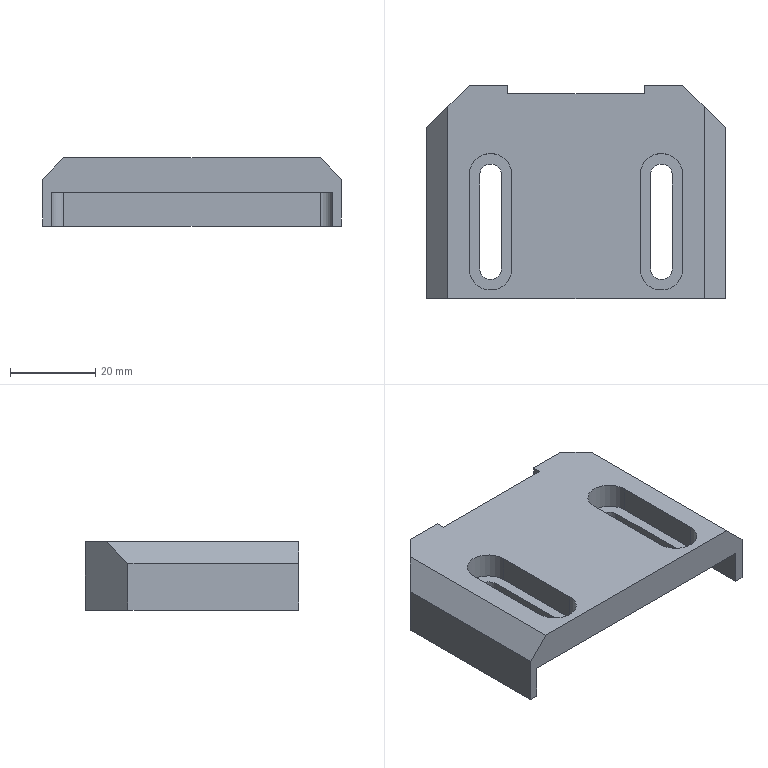Part | SolidWorks | features ICE 4, Chamfer 2, Extrusion 1, HoleWzd 1 | 1 solid | 46 faces | box 70 x 50 x 16 mm | volume 29528 mm3 | plane 28 | cylinder 14 | cone 4 | commonest cylinder face diameters 4.2 x4 5.1 x4 10 x4 6 x2
STEP:
#1=CARTESIAN_POINT('',(-10.,14.6,-2.1));
#2=VERTEX_POINT('',#1);
#3=CARTESIAN_POINT('',(-10.,14.6,2.1));
#4=VERTEX_POINT('',#3);
#5=CARTESIAN_POINT('',(-10.,14.6,0.));
#6=DIRECTION('',(0.,1.,0.));
#7=DIRECTION('',(0.,0.,1.));
#8=AXIS2_PLACEMENT_3D('',#5,#6,#7);
#9=CIRCLE('',#8,2.1);
#10=EDGE_CURVE('',#2,#4,#9,.T.);
#11=ORIENTED_EDGE('',*,*,#10,.F.);
#12=CARTESIAN_POINT('',(-10.,23.,-2.1));
#13=VERTEX_POINT('',#12);
#14=CARTESIAN_POINT('',(-10.,23.,-2.1));
#15=DIRECTION('',(0.,1.,0.));
#16=VECTOR('',#15,1000.);
#17=LINE('',#14,#16);
#18=EDGE_CURVE('',#2,#13,#17,.T.);
#19=ORIENTED_EDGE('',*,*,#18,.T.);
#20=CARTESIAN_POINT('',(-10.,23.,2.1));
#21=VERTEX_POINT('',#20);
#22=CARTESIAN_POINT('',(-10.,23.,0.));
#23=DIRECTION('',(0.,1.,0.));
#24=DIRECTION('',(0.,0.,1.));
#25=AXIS2_PLACEMENT_3D('',#22,#23,#24);
#26=CIRCLE('',#25,2.1);
#27=EDGE_CURVE('',#13,#21,#26,.T.);
#28=ORIENTED_EDGE('',*,*,#27,.T.);
#29=CARTESIAN_POINT('',(-10.,23.,2.1));
#30=DIRECTION('',(0.,1.,0.));
#31=VECTOR('',#30,1000.);
#32=LINE('',#29,#31);
#33=EDGE_CURVE('',#4,#21,#32,.T.);
#34=ORIENTED_EDGE('',*,*,#33,.F.);
#35=EDGE_LOOP('',(#11,#19,#28,#34));
#36=FACE_OUTER_BOUND('',#35,.T.);
#37=CARTESIAN_POINT('',(-10.,23.,0.));
#38=DIRECTION('',(0.,1.,0.));
#39=DIRECTION('',(0.,0.,1.));
#40=AXIS2_PLACEMENT_3D('',#37,#38,#39);
#41=CYLINDRICAL_SURFACE('',#40,2.1);
#42=ADVANCED_FACE('',(#36),#41,.F.);
#43=CARTESIAN_POINT('',(-10.,13.338,0.));
#44=VERTEX_POINT('',#43);
#45=CARTESIAN_POINT('',(-10.,14.6,2.1));
#46=DIRECTION('',(0.,0.515,0.8572));
#47=VECTOR('',#46,1000.);
#48=LINE('',#45,#47);
#49=EDGE_CURVE('',#44,#4,#48,.T.);
#50=ORIENTED_EDGE('',*,*,#49,.F.);
#51=CARTESIAN_POINT('',(-10.,14.6,-2.1));
#52=DIRECTION('',(0.,0.515,-0.8572));
#53=VECTOR('',#52,1000.);
#54=LINE('',#51,#53);
#55=EDGE_CURVE('',#44,#2,#54,.T.);
#56=ORIENTED_EDGE('',*,*,#55,.T.);
#57=ORIENTED_EDGE('',*,*,#10,.T.);
#58=EDGE_LOOP('',(#50,#56,#57));
#59=FACE_OUTER_BOUND('',#58,.T.);
#60=CARTESIAN_POINT('',(-10.,14.6,0.));
#61=DIRECTION('',(0.,1.,0.));
#62=DIRECTION('',(0.,0.,1.));
#63=AXIS2_PLACEMENT_3D('',#60,#61,#62);
#64=CONICAL_SURFACE('',#63,2.1,1.03);
#65=ADVANCED_FACE('',(#59),#64,.F.);
#66=CARTESIAN_POINT('',(10.,14.6,-2.1));
#67=VERTEX_POINT('',#66);
#68=CARTESIAN_POINT('',(10.,14.6,2.1));
#69=VERTEX_POINT('',#68);
#70=CARTESIAN_POINT('',(10.,14.6,0.));
#71=DIRECTION('',(0.,1.,0.));
#72=DIRECTION('',(0.,0.,1.));
#73=AXIS2_PLACEMENT_3D('',#70,#71,#72);
#74=CIRCLE('',#73,2.1);
#75=EDGE_CURVE('',#67,#69,#74,.T.);
#76=ORIENTED_EDGE('',*,*,#75,.F.);
#77=CARTESIAN_POINT('',(10.,23.,-2.1));
#78=VERTEX_POINT('',#77);
#79=CARTESIAN_POINT('',(10.,23.,-2.1));
#80=DIRECTION('',(0.,1.,0.));
#81=VECTOR('',#80,1000.);
#82=LINE('',#79,#81);
#83=EDGE_CURVE('',#67,#78,#82,.T.);
#84=ORIENTED_EDGE('',*,*,#83,.T.);
#85=CARTESIAN_POINT('',(10.,23.,2.1));
#86=VERTEX_POINT('',#85);
#87=CARTESIAN_POINT('',(10.,23.,0.));
#88=DIRECTION('',(0.,1.,0.));
#89=DIRECTION('',(0.,0.,1.));
#90=AXIS2_PLACEMENT_3D('',#87,#88,#89);
#91=CIRCLE('',#90,2.1);
#92=EDGE_CURVE('',#78,#86,#91,.T.);
#93=ORIENTED_EDGE('',*,*,#92,.T.);
#94=CARTESIAN_POINT('',(10.,23.,2.1));
#95=DIRECTION('',(0.,1.,0.));
#96=VECTOR('',#95,1000.);
#97=LINE('',#94,#96);
#98=EDGE_CURVE('',#69,#86,#97,.T.);
#99=ORIENTED_EDGE('',*,*,#98,.F.);
#100=EDGE_LOOP('',(#76,#84,#93,#99));
#101=FACE_OUTER_BOUND('',#100,.T.);
#102=CARTESIAN_POINT('',(10.,23.,0.));
#103=DIRECTION('',(0.,1.,0.));
#104=DIRECTION('',(0.,0.,1.));
#105=AXIS2_PLACEMENT_3D('',#102,#103,#104);
#106=CYLINDRICAL_SURFACE('',#105,2.1);
#107=ADVANCED_FACE('',(#101),#106,.F.);
#108=CARTESIAN_POINT('',(10.,13.338,0.));
#109=VERTEX_POINT('',#108);
#110=CARTESIAN_POINT('',(10.,14.6,2.1));
#111=DIRECTION('',(0.,0.515,0.8572));
#112=VECTOR('',#111,1000.);
#113=LINE('',#110,#112);
#114=EDGE_CURVE('',#109,#69,#113,.T.);
#115=ORIENTED_EDGE('',*,*,#114,.F.);
#116=CARTESIAN_POINT('',(10.,14.6,-2.1));
#117=DIRECTION('',(0.,0.515,-0.8572));
#118=VECTOR('',#117,1000.);
#119=LINE('',#116,#118);
#120=EDGE_CURVE('',#109,#67,#119,.T.);
#121=ORIENTED_EDGE('',*,*,#120,.T.);
#122=ORIENTED_EDGE('',*,*,#75,.T.);
#123=EDGE_LOOP('',(#115,#121,#122));
#124=FACE_OUTER_BOUND('',#123,.T.);
#125=CARTESIAN_POINT('',(10.,14.6,0.));
#126=DIRECTION('',(0.,1.,0.));
#127=DIRECTION('',(0.,0.,1.));
#128=AXIS2_PLACEMENT_3D('',#125,#126,#127);
#129=CONICAL_SURFACE('',#128,2.1,1.03);
#130=ADVANCED_FACE('',(#124),#129,.F.);
#131=CARTESIAN_POINT('',(-17.45,-18.,2.));
#132=VERTEX_POINT('',#131);
#133=CARTESIAN_POINT('',(-22.55,-18.,2.));
#134=VERTEX_POINT('',#133);
#135=CARTESIAN_POINT('',(-20.,-18.,2.));
#136=DIRECTION('',(0.,0.,-1.));
#137=DIRECTION('',(1.,0.,0.));
#138=AXIS2_PLACEMENT_3D('',#135,#136,#137);
#139=CIRCLE('',#138,2.55);
#140=EDGE_CURVE('',#132,#134,#139,.T.);
#141=ORIENTED_EDGE('',*,*,#140,.F.);
#142=CARTESIAN_POINT('',(-17.45,-18.,0.));
#143=VERTEX_POINT('',#142);
#144=CARTESIAN_POINT('',(-17.45,-18.,-8.));
#145=DIRECTION('',(0.,0.,1.));
#146=VECTOR('',#145,1000.);
#147=LINE('',#144,#146);
#148=EDGE_CURVE('',#143,#132,#147,.T.);
#149=ORIENTED_EDGE('',*,*,#148,.F.);
#150=CARTESIAN_POINT('',(-22.55,-18.,0.));
#151=VERTEX_POINT('',#150);
#152=CARTESIAN_POINT('',(-20.,-18.,0.));
#153=DIRECTION('',(0.,0.,-1.));
#154=DIRECTION('',(-1.,0.,0.));
#155=AXIS2_PLACEMENT_3D('',#152,#153,#154);
#156=CIRCLE('',#155,2.55);
#157=EDGE_CURVE('',#143,#151,#156,.T.);
#158=ORIENTED_EDGE('',*,*,#157,.T.);
#159=CARTESIAN_POINT('',(-22.55,-18.,-8.));
#160=DIRECTION('',(0.,0.,1.));
#161=VECTOR('',#160,1000.);
#162=LINE('',#159,#161);
#163=EDGE_CURVE('',#151,#134,#162,.T.);
#164=ORIENTED_EDGE('',*,*,#163,.T.);
#165=EDGE_LOOP('',(#141,#149,#158,#164));
#166=FACE_OUTER_BOUND('',#165,.T.);
#167=CARTESIAN_POINT('',(-20.,-18.,-8.));
#168=DIRECTION('',(0.,0.,1.));
#169=DIRECTION('',(1.,0.,0.));
#170=AXIS2_PLACEMENT_3D('',#167,#168,#169);
#171=CYLINDRICAL_SURFACE('',#170,2.55);
#172=ADVANCED_FACE('',(#166),#171,.F.);
#173=CARTESIAN_POINT('',(-22.55,4.,2.));
#174=VERTEX_POINT('',#173);
#175=CARTESIAN_POINT('',(-22.55,-18.,2.));
#176=DIRECTION('',(0.,1.,0.));
#177=VECTOR('',#176,1000.);
#178=LINE('',#175,#177);
#179=EDGE_CURVE('',#134,#174,#178,.T.);
#180=ORIENTED_EDGE('',*,*,#179,.F.);
#181=ORIENTED_EDGE('',*,*,#163,.F.);
#182=CARTESIAN_POINT('',(-22.55,4.,0.));
#183=VERTEX_POINT('',#182);
#184=CARTESIAN_POINT('',(-22.55,7.,0.));
#185=DIRECTION('',(0.,1.,0.));
#186=VECTOR('',#185,1000.);
#187=LINE('',#184,#186);
#188=EDGE_CURVE('',#151,#183,#187,.T.);
#189=ORIENTED_EDGE('',*,*,#188,.T.);
#190=CARTESIAN_POINT('',(-22.55,4.,-8.));
#191=DIRECTION('',(0.,0.,1.));
#192=VECTOR('',#191,1000.);
#193=LINE('',#190,#192);
#194=EDGE_CURVE('',#183,#174,#193,.T.);
#195=ORIENTED_EDGE('',*,*,#194,.T.);
#196=EDGE_LOOP('',(#180,#181,#189,#195));
#197=FACE_OUTER_BOUND('',#196,.T.);
#198=CARTESIAN_POINT('',(-22.55,-18.,-8.));
#199=DIRECTION('',(-1.,0.,0.));
#200=DIRECTION('',(0.,-1.,0.));
#201=AXIS2_PLACEMENT_3D('',#198,#199,#200);
#202=PLANE('',#201);
#203=ADVANCED_FACE('',(#197),#202,.F.);
#204=CARTESIAN_POINT('',(-17.45,4.,2.));
#205=VERTEX_POINT('',#204);
#206=CARTESIAN_POINT('',(-20.,4.,2.));
#207=DIRECTION('',(0.,0.,-1.));
#208=DIRECTION('',(1.,0.,0.));
#209=AXIS2_PLACEMENT_3D('',#206,#207,#208);
#210=CIRCLE('',#209,2.55);
#211=EDGE_CURVE('',#174,#205,#210,.T.);
#212=ORIENTED_EDGE('',*,*,#211,.F.);
#213=ORIENTED_EDGE('',*,*,#194,.F.);
#214=CARTESIAN_POINT('',(-17.45,4.,0.));
#215=VERTEX_POINT('',#214);
#216=CARTESIAN_POINT('',(-20.,4.,0.));
#217=DIRECTION('',(0.,0.,-1.));
#218=DIRECTION('',(-1.,0.,0.));
#219=AXIS2_PLACEMENT_3D('',#216,#217,#218);
#220=CIRCLE('',#219,2.55);
#221=EDGE_CURVE('',#183,#215,#220,.T.);
#222=ORIENTED_EDGE('',*,*,#221,.T.);
#223=CARTESIAN_POINT('',(-17.45,4.,-8.));
#224=DIRECTION('',(0.,0.,1.));
#225=VECTOR('',#224,1000.);
#226=LINE('',#223,#225);
#227=EDGE_CURVE('',#215,#205,#226,.T.);
#228=ORIENTED_EDGE('',*,*,#227,.T.);
#229=EDGE_LOOP('',(#212,#213,#222,#228));
#230=FACE_OUTER_BOUND('',#229,.T.);
#231=CARTESIAN_POINT('',(-20.,4.,-8.));
#232=DIRECTION('',(0.,0.,1.));
#233=DIRECTION('',(1.,0.,0.));
#234=AXIS2_PLACEMENT_3D('',#231,#232,#233);
#235=CYLINDRICAL_SURFACE('',#234,2.55);
#236=ADVANCED_FACE('',(#230),#235,.F.);
#237=CARTESIAN_POINT('',(-17.45,-18.,2.));
#238=DIRECTION('',(0.,-1.,0.));
#239=VECTOR('',#238,1000.);
#240=LINE('',#237,#239);
#241=EDGE_CURVE('',#205,#132,#240,.T.);
#242=ORIENTED_EDGE('',*,*,#241,.F.);
#243=ORIENTED_EDGE('',*,*,#227,.F.);
#244=CARTESIAN_POINT('',(-17.45,7.,0.));
#245=DIRECTION('',(0.,-1.,0.));
#246=VECTOR('',#245,1000.);
#247=LINE('',#244,#246);
#248=EDGE_CURVE('',#215,#143,#247,.T.);
#249=ORIENTED_EDGE('',*,*,#248,.T.);
#250=ORIENTED_EDGE('',*,*,#148,.T.);
#251=EDGE_LOOP('',(#242,#243,#249,#250));
#252=FACE_OUTER_BOUND('',#251,.T.);
#253=CARTESIAN_POINT('',(-17.45,-18.,-8.));
#254=DIRECTION('',(1.,0.,0.));
#255=DIRECTION('',(0.,1.,0.));
#256=AXIS2_PLACEMENT_3D('',#253,#254,#255);
#257=PLANE('',#256);
#258=ADVANCED_FACE('',(#252),#257,.F.);
#259=CARTESIAN_POINT('',(22.55,-18.,2.));
#260=VERTEX_POINT('',#259);
#261=CARTESIAN_POINT('',(17.45,-18.,2.));
#262=VERTEX_POINT('',#261);
#263=CARTESIAN_POINT('',(20.,-18.,2.));
#264=DIRECTION('',(0.,0.,-1.));
#265=DIRECTION('',(1.,0.,0.));
#266=AXIS2_PLACEMENT_3D('',#263,#264,#265);
#267=CIRCLE('',#266,2.55);
#268=EDGE_CURVE('',#260,#262,#267,.T.);
#269=ORIENTED_EDGE('',*,*,#268,.F.);
#270=CARTESIAN_POINT('',(22.55,-18.,0.));
#271=VERTEX_POINT('',#270);
#272=CARTESIAN_POINT('',(22.55,-18.,-8.));
#273=DIRECTION('',(0.,0.,1.));
#274=VECTOR('',#273,1000.);
#275=LINE('',#272,#274);
#276=EDGE_CURVE('',#271,#260,#275,.T.);
#277=ORIENTED_EDGE('',*,*,#276,.F.);
#278=CARTESIAN_POINT('',(17.45,-18.,0.));
#279=VERTEX_POINT('',#278);
#280=CARTESIAN_POINT('',(20.,-18.,0.));
#281=DIRECTION('',(0.,0.,-1.));
#282=DIRECTION('',(-1.,0.,0.));
#283=AXIS2_PLACEMENT_3D('',#280,#281,#282);
#284=CIRCLE('',#283,2.55);
#285=EDGE_CURVE('',#271,#279,#284,.T.);
#286=ORIENTED_EDGE('',*,*,#285,.T.);
#287=CARTESIAN_POINT('',(17.45,-18.,-8.));
#288=DIRECTION('',(0.,0.,1.));
#289=VECTOR('',#288,1000.);
#290=LINE('',#287,#289);
#291=EDGE_CURVE('',#279,#262,#290,.T.);
#292=ORIENTED_EDGE('',*,*,#291,.T.);
#293=EDGE_LOOP('',(#269,#277,#286,#292));
#294=FACE_OUTER_BOUND('',#293,.T.);
#295=CARTESIAN_POINT('',(20.,-18.,-8.));
#296=DIRECTION('',(0.,0.,1.));
#297=DIRECTION('',(1.,0.,0.));
#298=AXIS2_PLACEMENT_3D('',#295,#296,#297);
#299=CYLINDRICAL_SURFACE('',#298,2.55);
#300=ADVANCED_FACE('',(#294),#299,.F.);
#301=CARTESIAN_POINT('',(17.45,4.,2.));
#302=VERTEX_POINT('',#301);
#303=CARTESIAN_POINT('',(17.45,-18.,2.));
#304=DIRECTION('',(0.,1.,0.));
#305=VECTOR('',#304,1000.);
#306=LINE('',#303,#305);
#307=EDGE_CURVE('',#262,#302,#306,.T.);
#308=ORIENTED_EDGE('',*,*,#307,.F.);
#309=ORIENTED_EDGE('',*,*,#291,.F.);
#310=CARTESIAN_POINT('',(17.45,4.,0.));
#311=VERTEX_POINT('',#310);
#312=CARTESIAN_POINT('',(17.45,7.,0.));
#313=DIRECTION('',(0.,1.,0.));
#314=VECTOR('',#313,1000.);
#315=LINE('',#312,#314);
#316=EDGE_CURVE('',#279,#311,#315,.T.);
#317=ORIENTED_EDGE('',*,*,#316,.T.);
#318=CARTESIAN_POINT('',(17.45,4.,-8.));
#319=DIRECTION('',(0.,0.,1.));
#320=VECTOR('',#319,1000.);
#321=LINE('',#318,#320);
#322=EDGE_CURVE('',#311,#302,#321,.T.);
#323=ORIENTED_EDGE('',*,*,#322,.T.);
#324=EDGE_LOOP('',(#308,#309,#317,#323));
#325=FACE_OUTER_BOUND('',#324,.T.);
#326=CARTESIAN_POINT('',(17.45,-18.,-8.));
#327=DIRECTION('',(-1.,0.,0.));
#328=DIRECTION('',(0.,0.,1.));
#329=AXIS2_PLACEMENT_3D('',#326,#327,#328);
#330=PLANE('',#329);
#331=ADVANCED_FACE('',(#325),#330,.F.);
#332=CARTESIAN_POINT('',(22.55,4.,2.));
#333=VERTEX_POINT('',#332);
#334=CARTESIAN_POINT('',(20.,4.,2.));
#335=DIRECTION('',(0.,0.,-1.));
#336=DIRECTION('',(1.,0.,0.));
#337=AXIS2_PLACEMENT_3D('',#334,#335,#336);
#338=CIRCLE('',#337,2.55);
#339=EDGE_CURVE('',#302,#333,#338,.T.);
#340=ORIENTED_EDGE('',*,*,#339,.F.);
#341=ORIENTED_EDGE('',*,*,#322,.F.);
#342=CARTESIAN_POINT('',(22.55,4.,0.));
#343=VERTEX_POINT('',#342);
#344=CARTESIAN_POINT('',(20.,4.,0.));
#345=DIRECTION('',(0.,0.,-1.));
#346=DIRECTION('',(-1.,0.,0.));
#347=AXIS2_PLACEMENT_3D('',#344,#345,#346);
#348=CIRCLE('',#347,2.55);
#349=EDGE_CURVE('',#311,#343,#348,.T.);
#350=ORIENTED_EDGE('',*,*,#349,.T.);
#351=CARTESIAN_POINT('',(22.55,4.,-8.));
#352=DIRECTION('',(0.,0.,1.));
#353=VECTOR('',#352,1000.);
#354=LINE('',#351,#353);
#355=EDGE_CURVE('',#343,#333,#354,.T.);
#356=ORIENTED_EDGE('',*,*,#355,.T.);
#357=EDGE_LOOP('',(#340,#341,#350,#356));
#358=FACE_OUTER_BOUND('',#357,.T.);
#359=CARTESIAN_POINT('',(20.,4.,-8.));
#360=DIRECTION('',(0.,0.,1.));
#361=DIRECTION('',(1.,0.,0.));
#362=AXIS2_PLACEMENT_3D('',#359,#360,#361);
#363=CYLINDRICAL_SURFACE('',#362,2.55);
#364=ADVANCED_FACE('',(#358),#363,.F.);
#365=CARTESIAN_POINT('',(22.55,-18.,2.));
#366=DIRECTION('',(0.,-1.,0.));
#367=VECTOR('',#366,1000.);
#368=LINE('',#365,#367);
#369=EDGE_CURVE('',#333,#260,#368,.T.);
#370=ORIENTED_EDGE('',*,*,#369,.F.);
#371=ORIENTED_EDGE('',*,*,#355,.F.);
#372=CARTESIAN_POINT('',(22.55,7.,0.));
#373=DIRECTION('',(0.,-1.,0.));
#374=VECTOR('',#373,1000.);
#375=LINE('',#372,#374);
#376=EDGE_CURVE('',#343,#271,#375,.T.);
#377=ORIENTED_EDGE('',*,*,#376,.T.);
#378=ORIENTED_EDGE('',*,*,#276,.T.);
#379=EDGE_LOOP('',(#370,#371,#377,#378));
#380=FACE_OUTER_BOUND('',#379,.T.);
#381=CARTESIAN_POINT('',(22.55,-18.,-8.));
#382=DIRECTION('',(1.,0.,0.));
#383=DIRECTION('',(0.,0.,-1.));
#384=AXIS2_PLACEMENT_3D('',#381,#382,#383);
#385=PLANE('',#384);
#386=ADVANCED_FACE('',(#380),#385,.F.);
#387=CARTESIAN_POINT('',(-30.,-25.,8.));
#388=VERTEX_POINT('',#387);
#389=CARTESIAN_POINT('',(30.,-25.,8.));
#390=VERTEX_POINT('',#389);
#391=CARTESIAN_POINT('',(35.,-25.,8.));
#392=DIRECTION('',(1.,0.,0.));
#393=VECTOR('',#392,1000.);
#394=LINE('',#391,#393);
#395=EDGE_CURVE('',#388,#390,#394,.T.);
#396=ORIENTED_EDGE('',*,*,#395,.F.);
#397=CARTESIAN_POINT('',(-35.,-25.,3.));
#398=VERTEX_POINT('',#397);
#399=CARTESIAN_POINT('',(-30.,-25.,8.));
#400=DIRECTION('',(-0.7071,0.,-0.7071));
#401=VECTOR('',#400,1000.);
#402=LINE('',#399,#401);
#403=EDGE_CURVE('',#388,#398,#402,.T.);
#404=ORIENTED_EDGE('',*,*,#403,.T.);
#405=CARTESIAN_POINT('',(-35.,-25.,-8.));
#406=VERTEX_POINT('',#405);
#407=CARTESIAN_POINT('',(-35.,-25.,8.));
#408=DIRECTION('',(0.,0.,-1.));
#409=VECTOR('',#408,1000.);
#410=LINE('',#407,#409);
#411=EDGE_CURVE('',#398,#406,#410,.T.);
#412=ORIENTED_EDGE('',*,*,#411,.T.);
#413=CARTESIAN_POINT('',(-33.,-25.,-8.));
#414=VERTEX_POINT('',#413);
#415=CARTESIAN_POINT('',(35.,-25.,-8.));
#416=DIRECTION('',(1.,0.,0.));
#417=VECTOR('',#416,1000.);
#418=LINE('',#415,#417);
#419=EDGE_CURVE('',#406,#414,#418,.T.);
#420=ORIENTED_EDGE('',*,*,#419,.T.);
#421=CARTESIAN_POINT('',(-33.,-25.,0.));
#422=VERTEX_POINT('',#421);
#423=CARTESIAN_POINT('',(-33.,-25.,0.));
#424=DIRECTION('',(0.,0.,-1.));
#425=VECTOR('',#424,1000.);
#426=LINE('',#423,#425);
#427=EDGE_CURVE('',#422,#414,#426,.T.);
#428=ORIENTED_EDGE('',*,*,#427,.F.);
#429=CARTESIAN_POINT('',(33.,-25.,0.));
#430=VERTEX_POINT('',#429);
#431=CARTESIAN_POINT('',(-33.,-25.,0.));
#432=DIRECTION('',(1.,0.,0.));
#433=VECTOR('',#432,1000.);
#434=LINE('',#431,#433);
#435=EDGE_CURVE('',#422,#430,#434,.T.);
#436=ORIENTED_EDGE('',*,*,#435,.T.);
#437=CARTESIAN_POINT('',(33.,-25.,-8.));
#438=VERTEX_POINT('',#437);
#439=CARTESIAN_POINT('',(33.,-25.,0.));
#440=DIRECTION('',(0.,0.,-1.));
#441=VECTOR('',#440,1000.);
#442=LINE('',#439,#441);
#443=EDGE_CURVE('',#430,#438,#442,.T.);
#444=ORIENTED_EDGE('',*,*,#443,.T.);
#445=CARTESIAN_POINT('',(35.,-25.,-8.));
#446=VERTEX_POINT('',#445);
#447=CARTESIAN_POINT('',(35.,-25.,-8.));
#448=DIRECTION('',(1.,0.,0.));
#449=VECTOR('',#448,1000.);
#450=LINE('',#447,#449);
#451=EDGE_CURVE('',#438,#446,#450,.T.);
#452=ORIENTED_EDGE('',*,*,#451,.T.);
#453=CARTESIAN_POINT('',(35.,-25.,3.));
#454=VERTEX_POINT('',#453);
#455=CARTESIAN_POINT('',(35.,-25.,8.));
#456=DIRECTION('',(0.,0.,-1.));
#457=VECTOR('',#456,1000.);
#458=LINE('',#455,#457);
#459=EDGE_CURVE('',#454,#446,#458,.T.);
#460=ORIENTED_EDGE('',*,*,#459,.F.);
#461=CARTESIAN_POINT('',(30.,-25.,8.));
#462=DIRECTION('',(-0.7071,0.,0.7071));
#463=VECTOR('',#462,1000.);
#464=LINE('',#461,#463);
#465=EDGE_CURVE('',#454,#390,#464,.T.);
#466=ORIENTED_EDGE('',*,*,#465,.T.);
#467=EDGE_LOOP('',(#396,#404,#412,#420,#428,#436,#444,#452,#460,#466));
#468=FACE_OUTER_BOUND('',#467,.T.);
#469=CARTESIAN_POINT('',(35.,-25.,8.));
#470=DIRECTION('',(0.,1.,0.));
#471=DIRECTION('',(-1.,0.,0.));
#472=AXIS2_PLACEMENT_3D('',#469,#470,#471);
#473=PLANE('',#472);
#474=ADVANCED_FACE('',(#468),#473,.F.);
#475=CARTESIAN_POINT('',(-35.,15.,-8.));
#476=VERTEX_POINT('',#475);
#477=CARTESIAN_POINT('',(-35.,-25.,-8.));
#478=DIRECTION('',(0.,-1.,0.));
#479=VECTOR('',#478,1000.);
#480=LINE('',#477,#479);
#481=EDGE_CURVE('',#476,#406,#480,.T.);
#482=ORIENTED_EDGE('',*,*,#481,.F.);
#483=CARTESIAN_POINT('',(-25.,25.,-8.));
#484=VERTEX_POINT('',#483);
#485=CARTESIAN_POINT('',(-35.,15.,-8.));
#486=DIRECTION('',(0.7071,0.7071,0.));
#487=VECTOR('',#486,1000.);
#488=LINE('',#485,#487);
#489=EDGE_CURVE('',#476,#484,#488,.T.);
#490=ORIENTED_EDGE('',*,*,#489,.T.);
#491=CARTESIAN_POINT('',(-16.,25.,-8.));
#492=VERTEX_POINT('',#491);
#493=CARTESIAN_POINT('',(35.,25.,-8.));
#494=DIRECTION('',(-1.,0.,0.));
#495=VECTOR('',#494,1000.);
#496=LINE('',#493,#495);
#497=EDGE_CURVE('',#492,#484,#496,.T.);
#498=ORIENTED_EDGE('',*,*,#497,.F.);
#499=CARTESIAN_POINT('',(-16.,23.,-8.));
#500=VERTEX_POINT('',#499);
#501=CARTESIAN_POINT('',(-16.,23.,-8.));
#502=DIRECTION('',(0.,1.,0.));
#503=VECTOR('',#502,1000.);
#504=LINE('',#501,#503);
#505=EDGE_CURVE('',#500,#492,#504,.T.);
#506=ORIENTED_EDGE('',*,*,#505,.F.);
#507=CARTESIAN_POINT('',(16.,23.,-8.));
#508=VERTEX_POINT('',#507);
#509=CARTESIAN_POINT('',(16.,23.,-8.));
#510=DIRECTION('',(-1.,0.,0.));
#511=VECTOR('',#510,1000.);
#512=LINE('',#509,#511);
#513=EDGE_CURVE('',#508,#500,#512,.T.);
#514=ORIENTED_EDGE('',*,*,#513,.F.);
#515=CARTESIAN_POINT('',(16.,25.,-8.));
#516=VERTEX_POINT('',#515);
#517=CARTESIAN_POINT('',(16.,23.,-8.));
#518=DIRECTION('',(0.,1.,0.));
#519=VECTOR('',#518,1000.);
#520=LINE('',#517,#519);
#521=EDGE_CURVE('',#508,#516,#520,.T.);
#522=ORIENTED_EDGE('',*,*,#521,.T.);
#523=CARTESIAN_POINT('',(25.,25.,-8.));
#524=VERTEX_POINT('',#523);
#525=CARTESIAN_POINT('',(35.,25.,-8.));
#526=DIRECTION('',(-1.,0.,0.));
#527=VECTOR('',#526,1000.);
#528=LINE('',#525,#527);
#529=EDGE_CURVE('',#524,#516,#528,.T.);
#530=ORIENTED_EDGE('',*,*,#529,.F.);
#531=CARTESIAN_POINT('',(35.,15.,-8.));
#532=VERTEX_POINT('',#531);
#533=CARTESIAN_POINT('',(25.,25.,-8.));
#534=DIRECTION('',(0.7071,-0.7071,0.));
#535=VECTOR('',#534,1000.);
#536=LINE('',#533,#535);
#537=EDGE_CURVE('',#524,#532,#536,.T.);
#538=ORIENTED_EDGE('',*,*,#537,.T.);
#539=CARTESIAN_POINT('',(35.,-25.,-8.));
#540=DIRECTION('',(0.,1.,0.));
#541=VECTOR('',#540,1000.);
#542=LINE('',#539,#541);
#543=EDGE_CURVE('',#446,#532,#542,.T.);
#544=ORIENTED_EDGE('',*,*,#543,.F.);
#545=ORIENTED_EDGE('',*,*,#451,.F.);
#546=CARTESIAN_POINT('',(33.,7.,-8.));
#547=VERTEX_POINT('',#546);
#548=CARTESIAN_POINT('',(33.,-25.,-8.));
#549=DIRECTION('',(0.,1.,0.));
#550=VECTOR('',#549,1000.);
#551=LINE('',#548,#550);
#552=EDGE_CURVE('',#438,#547,#551,.T.);
#553=ORIENTED_EDGE('',*,*,#552,.T.);
#554=CARTESIAN_POINT('',(30.,10.,-8.));
#555=VERTEX_POINT('',#554);
#556=CARTESIAN_POINT('',(30.,7.,-8.));
#557=DIRECTION('',(0.,0.,1.));
#558=DIRECTION('',(-1.,0.,0.));
#559=AXIS2_PLACEMENT_3D('',#556,#557,#558);
#560=CIRCLE('',#559,3.);
#561=EDGE_CURVE('',#547,#555,#560,.T.);
#562=ORIENTED_EDGE('',*,*,#561,.T.);
#563=CARTESIAN_POINT('',(-30.,10.,-8.));
#564=VERTEX_POINT('',#563);
#565=CARTESIAN_POINT('',(-30.,10.,-8.));
#566=DIRECTION('',(-1.,0.,0.));
#567=VECTOR('',#566,1000.);
#568=LINE('',#565,#567);
#569=EDGE_CURVE('',#555,#564,#568,.T.);
#570=ORIENTED_EDGE('',*,*,#569,.T.);
#571=CARTESIAN_POINT('',(-33.,7.,-8.));
#572=VERTEX_POINT('',#571);
#573=CARTESIAN_POINT('',(-30.,7.,-8.));
#574=DIRECTION('',(0.,0.,1.));
#575=DIRECTION('',(-1.,0.,0.));
#576=AXIS2_PLACEMENT_3D('',#573,#574,#575);
#577=CIRCLE('',#576,3.);
#578=EDGE_CURVE('',#564,#572,#577,.T.);
#579=ORIENTED_EDGE('',*,*,#578,.T.);
#580=CARTESIAN_POINT('',(-33.,-25.,-8.));
#581=DIRECTION('',(0.,-1.,0.));
#582=VECTOR('',#581,1000.);
#583=LINE('',#580,#582);
#584=EDGE_CURVE('',#572,#414,#583,.T.);
#585=ORIENTED_EDGE('',*,*,#584,.T.);
#586=ORIENTED_EDGE('',*,*,#419,.F.);
#587=EDGE_LOOP('',(#482,#490,#498,#506,#514,#522,#530,#538,#544,#545,#553,#562,#570,#579,#585,#586));
#588=FACE_OUTER_BOUND('',#587,.T.);
#589=CARTESIAN_POINT('',(0.,0.,-8.));
#590=DIRECTION('',(0.,0.,1.));
#591=DIRECTION('',(1.,0.,0.));
#592=AXIS2_PLACEMENT_3D('',#589,#590,#591);
#593=PLANE('',#592);
#594=ADVANCED_FACE('',(#588),#593,.F.);
#595=ORIENTED_EDGE('',*,*,#497,.T.);
#596=CARTESIAN_POINT('',(-25.,25.,8.));
#597=VERTEX_POINT('',#596);
#598=CARTESIAN_POINT('',(-25.,25.,8.));
#599=DIRECTION('',(0.,0.,1.));
#600=VECTOR('',#599,1000.);
#601=LINE('',#598,#600);
#602=EDGE_CURVE('',#484,#597,#601,.T.);
#603=ORIENTED_EDGE('',*,*,#602,.T.);
#604=CARTESIAN_POINT('',(-16.,25.,8.));
#605=VERTEX_POINT('',#604);
#606=CARTESIAN_POINT('',(35.,25.,8.));
#607=DIRECTION('',(-1.,0.,0.));
#608=VECTOR('',#607,1000.);
#609=LINE('',#606,#608);
#610=EDGE_CURVE('',#605,#597,#609,.T.);
#611=ORIENTED_EDGE('',*,*,#610,.F.);
#612=CARTESIAN_POINT('',(-16.,25.,8.));
#613=DIRECTION('',(0.,0.,1.));
#614=VECTOR('',#613,1000.);
#615=LINE('',#612,#614);
#616=EDGE_CURVE('',#492,#605,#615,.T.);
#617=ORIENTED_EDGE('',*,*,#616,.F.);
#618=EDGE_LOOP('',(#595,#603,#611,#617));
#619=FACE_OUTER_BOUND('',#618,.T.);
#620=CARTESIAN_POINT('',(35.,25.,8.));
#621=DIRECTION('',(0.,-1.,0.));
#622=DIRECTION('',(1.,0.,0.));
#623=AXIS2_PLACEMENT_3D('',#620,#621,#622);
#624=PLANE('',#623);
#625=ADVANCED_FACE('',(#619),#624,.F.);
#626=ORIENTED_EDGE('',*,*,#411,.F.);
#627=CARTESIAN_POINT('',(-35.,15.,3.));
#628=VERTEX_POINT('',#627);
#629=CARTESIAN_POINT('',(-35.,15.,3.));
#630=DIRECTION('',(0.,1.,0.));
#631=VECTOR('',#630,1000.);
#632=LINE('',#629,#631);
#633=EDGE_CURVE('',#398,#628,#632,.T.);
#634=ORIENTED_EDGE('',*,*,#633,.T.);
#635=CARTESIAN_POINT('',(-35.,15.,8.));
#636=DIRECTION('',(0.,0.,-1.));
#637=VECTOR('',#636,1000.);
#638=LINE('',#635,#637);
#639=EDGE_CURVE('',#628,#476,#638,.T.);
#640=ORIENTED_EDGE('',*,*,#639,.T.);
#641=ORIENTED_EDGE('',*,*,#481,.T.);
#642=EDGE_LOOP('',(#626,#634,#640,#641));
#643=FACE_OUTER_BOUND('',#642,.T.);
#644=CARTESIAN_POINT('',(-35.,-25.,8.));
#645=DIRECTION('',(1.,0.,0.));
#646=DIRECTION('',(0.,0.,-1.));
#647=AXIS2_PLACEMENT_3D('',#644,#645,#646);
#648=PLANE('',#647);
#649=ADVANCED_FACE('',(#643),#648,.F.);
#650=CARTESIAN_POINT('',(35.,15.,3.));
#651=VERTEX_POINT('',#650);
#652=CARTESIAN_POINT('',(35.,15.,8.));
#653=DIRECTION('',(0.,0.,1.));
#654=VECTOR('',#653,1000.);
#655=LINE('',#652,#654);
#656=EDGE_CURVE('',#532,#651,#655,.T.);
#657=ORIENTED_EDGE('',*,*,#656,.T.);
#658=CARTESIAN_POINT('',(35.,-25.,3.));
#659=DIRECTION('',(0.,-1.,0.));
#660=VECTOR('',#659,1000.);
#661=LINE('',#658,#660);
#662=EDGE_CURVE('',#651,#454,#661,.T.);
#663=ORIENTED_EDGE('',*,*,#662,.T.);
#664=ORIENTED_EDGE('',*,*,#459,.T.);
#665=ORIENTED_EDGE('',*,*,#543,.T.);
#666=EDGE_LOOP('',(#657,#663,#664,#665));
#667=FACE_OUTER_BOUND('',#666,.T.);
#668=CARTESIAN_POINT('',(35.,-25.,8.));
#669=DIRECTION('',(-1.,0.,0.));
#670=DIRECTION('',(0.,0.,1.));
#671=AXIS2_PLACEMENT_3D('',#668,#669,#670);
#672=PLANE('',#671);
#673=ADVANCED_FACE('',(#667),#672,.F.);
#674=CARTESIAN_POINT('',(25.,25.,8.));
#675=VERTEX_POINT('',#674);
#676=CARTESIAN_POINT('',(16.,25.,8.));
#677=VERTEX_POINT('',#676);
#678=CARTESIAN_POINT('',(35.,25.,8.));
#679=DIRECTION('',(-1.,0.,0.));
#680=VECTOR('',#679,1000.);
#681=LINE('',#678,#680);
#682=EDGE_CURVE('',#675,#677,#681,.T.);
#683=ORIENTED_EDGE('',*,*,#682,.F.);
#684=CARTESIAN_POINT('',(25.,25.,8.));
#685=DIRECTION('',(0.,0.,-1.));
#686=VECTOR('',#685,1000.);
#687=LINE('',#684,#686);
#688=EDGE_CURVE('',#675,#524,#687,.T.);
#689=ORIENTED_EDGE('',*,*,#688,.T.);
#690=ORIENTED_EDGE('',*,*,#529,.T.);
#691=CARTESIAN_POINT('',(16.,25.,8.));
#692=DIRECTION('',(0.,0.,-1.));
#693=VECTOR('',#692,1000.);
#694=LINE('',#691,#693);
#695=EDGE_CURVE('',#677,#516,#694,.T.);
#696=ORIENTED_EDGE('',*,*,#695,.F.);
#697=EDGE_LOOP('',(#683,#689,#690,#696));
#698=FACE_OUTER_BOUND('',#697,.T.);
#699=CARTESIAN_POINT('',(35.,25.,8.));
#700=DIRECTION('',(0.,-1.,0.));
#701=DIRECTION('',(1.,0.,0.));
#702=AXIS2_PLACEMENT_3D('',#699,#700,#701);
#703=PLANE('',#702);
#704=ADVANCED_FACE('',(#698),#703,.F.);
#705=CARTESIAN_POINT('',(-15.,4.,8.));
#706=VERTEX_POINT('',#705);
#707=CARTESIAN_POINT('',(-25.,4.,8.));
#708=VERTEX_POINT('',#707);
#709=CARTESIAN_POINT('',(-20.,4.,8.));
#710=DIRECTION('',(0.,0.,1.));
#711=DIRECTION('',(1.,0.,0.));
#712=AXIS2_PLACEMENT_3D('',#709,#710,#711);
#713=CIRCLE('',#712,5.);
#714=EDGE_CURVE('',#706,#708,#713,.T.);
#715=ORIENTED_EDGE('',*,*,#714,.F.);
#716=CARTESIAN_POINT('',(-15.,-18.,8.));
#717=VERTEX_POINT('',#716);
#718=CARTESIAN_POINT('',(-15.,4.,8.));
#719=DIRECTION('',(0.,1.,0.));
#720=VECTOR('',#719,1000.);
#721=LINE('',#718,#720);
#722=EDGE_CURVE('',#717,#706,#721,.T.);
#723=ORIENTED_EDGE('',*,*,#722,.F.);
#724=CARTESIAN_POINT('',(-25.,-18.,8.));
#725=VERTEX_POINT('',#724);
#726=CARTESIAN_POINT('',(-20.,-18.,8.));
#727=DIRECTION('',(0.,0.,1.));
#728=DIRECTION('',(1.,0.,0.));
#729=AXIS2_PLACEMENT_3D('',#726,#727,#728);
#730=CIRCLE('',#729,5.);
#731=EDGE_CURVE('',#725,#717,#730,.T.);
#732=ORIENTED_EDGE('',*,*,#731,.F.);
#733=CARTESIAN_POINT('',(-25.,4.,8.));
#734=DIRECTION('',(0.,-1.,0.));
#735=VECTOR('',#734,1000.);
#736=LINE('',#733,#735);
#737=EDGE_CURVE('',#708,#725,#736,.T.);
#738=ORIENTED_EDGE('',*,*,#737,.F.);
#739=EDGE_LOOP('',(#715,#723,#732,#738));
#740=FACE_BOUND('',#739,.T.);
#741=CARTESIAN_POINT('',(15.,-18.,8.));
#742=VERTEX_POINT('',#741);
#743=CARTESIAN_POINT('',(25.,-18.,8.));
#744=VERTEX_POINT('',#743);
#745=CARTESIAN_POINT('',(20.,-18.,8.));
#746=DIRECTION('',(0.,0.,1.));
#747=DIRECTION('',(1.,0.,0.));
#748=AXIS2_PLACEMENT_3D('',#745,#746,#747);
#749=CIRCLE('',#748,5.);
#750=EDGE_CURVE('',#742,#744,#749,.T.);
#751=ORIENTED_EDGE('',*,*,#750,.F.);
#752=CARTESIAN_POINT('',(15.,4.,8.));
#753=VERTEX_POINT('',#752);
#754=CARTESIAN_POINT('',(15.,-18.,8.));
#755=DIRECTION('',(0.,-1.,0.));
#756=VECTOR('',#755,1000.);
#757=LINE('',#754,#756);
#758=EDGE_CURVE('',#753,#742,#757,.T.);
#759=ORIENTED_EDGE('',*,*,#758,.F.);
#760=CARTESIAN_POINT('',(25.,4.,8.));
#761=VERTEX_POINT('',#760);
#762=CARTESIAN_POINT('',(20.,4.,8.));
#763=DIRECTION('',(0.,0.,1.));
#764=DIRECTION('',(1.,0.,0.));
#765=AXIS2_PLACEMENT_3D('',#762,#763,#764);
#766=CIRCLE('',#765,5.);
#767=EDGE_CURVE('',#761,#753,#766,.T.);
#768=ORIENTED_EDGE('',*,*,#767,.F.);
#769=CARTESIAN_POINT('',(25.,-18.,8.));
#770=DIRECTION('',(0.,1.,0.));
#771=VECTOR('',#770,1000.);
#772=LINE('',#769,#771);
#773=EDGE_CURVE('',#744,#761,#772,.T.);
#774=ORIENTED_EDGE('',*,*,#773,.F.);
#775=EDGE_LOOP('',(#751,#759,#768,#774));
#776=FACE_BOUND('',#775,.T.);
#777=CARTESIAN_POINT('',(-30.,20.,8.));
#778=VERTEX_POINT('',#777);
#779=CARTESIAN_POINT('',(-25.,25.,8.));
#780=DIRECTION('',(-0.7071,-0.7071,0.));
#781=VECTOR('',#780,1000.);
#782=LINE('',#779,#781);
#783=EDGE_CURVE('',#597,#778,#782,.T.);
#784=ORIENTED_EDGE('',*,*,#783,.T.);
#785=CARTESIAN_POINT('',(-30.,-25.,8.));
#786=DIRECTION('',(0.,-1.,0.));
#787=VECTOR('',#786,1000.);
#788=LINE('',#785,#787);
#789=EDGE_CURVE('',#778,#388,#788,.T.);
#790=ORIENTED_EDGE('',*,*,#789,.T.);
#791=ORIENTED_EDGE('',*,*,#395,.T.);
#792=CARTESIAN_POINT('',(30.,20.,8.));
#793=VERTEX_POINT('',#792);
#794=CARTESIAN_POINT('',(30.,15.,8.));
#795=DIRECTION('',(0.,1.,0.));
#796=VECTOR('',#795,1000.);
#797=LINE('',#794,#796);
#798=EDGE_CURVE('',#390,#793,#797,.T.);
#799=ORIENTED_EDGE('',*,*,#798,.T.);
#800=CARTESIAN_POINT('',(25.,25.,8.));
#801=DIRECTION('',(-0.7071,0.7071,0.));
#802=VECTOR('',#801,1000.);
#803=LINE('',#800,#802);
#804=EDGE_CURVE('',#793,#675,#803,.T.);
#805=ORIENTED_EDGE('',*,*,#804,.T.);
#806=ORIENTED_EDGE('',*,*,#682,.T.);
#807=CARTESIAN_POINT('',(16.,23.,8.));
#808=VERTEX_POINT('',#807);
#809=CARTESIAN_POINT('',(16.,23.,8.));
#810=DIRECTION('',(0.,1.,0.));
#811=VECTOR('',#810,1000.);
#812=LINE('',#809,#811);
#813=EDGE_CURVE('',#808,#677,#812,.T.);
#814=ORIENTED_EDGE('',*,*,#813,.F.);
#815=CARTESIAN_POINT('',(-16.,23.,8.));
#816=VERTEX_POINT('',#815);
#817=CARTESIAN_POINT('',(16.,23.,8.));
#818=DIRECTION('',(1.,0.,0.));
#819=VECTOR('',#818,1000.);
#820=LINE('',#817,#819);
#821=EDGE_CURVE('',#816,#808,#820,.T.);
#822=ORIENTED_EDGE('',*,*,#821,.F.);
#823=CARTESIAN_POINT('',(-16.,23.,8.));
#824=DIRECTION('',(0.,1.,0.));
#825=VECTOR('',#824,1000.);
#826=LINE('',#823,#825);
#827=EDGE_CURVE('',#816,#605,#826,.T.);
#828=ORIENTED_EDGE('',*,*,#827,.T.);
#829=ORIENTED_EDGE('',*,*,#610,.T.);
#830=EDGE_LOOP('',(#784,#790,#791,#799,#805,#806,#814,#822,#828,#829));
#831=FACE_OUTER_BOUND('',#830,.T.);
#832=CARTESIAN_POINT('',(0.,0.,8.));
#833=DIRECTION('',(0.,0.,1.));
#834=DIRECTION('',(1.,0.,0.));
#835=AXIS2_PLACEMENT_3D('',#832,#833,#834);
#836=PLANE('',#835);
#837=ADVANCED_FACE('',(#740,#776,#831),#836,.T.);
#838=ORIENTED_EDGE('',*,*,#616,.T.);
#839=ORIENTED_EDGE('',*,*,#827,.F.);
#840=CARTESIAN_POINT('',(-16.,23.,8.));
#841=DIRECTION('',(0.,0.,1.));
#842=VECTOR('',#841,1000.);
#843=LINE('',#840,#842);
#844=EDGE_CURVE('',#500,#816,#843,.T.);
#845=ORIENTED_EDGE('',*,*,#844,.F.);
#846=ORIENTED_EDGE('',*,*,#505,.T.);
#847=EDGE_LOOP('',(#838,#839,#845,#846));
#848=FACE_OUTER_BOUND('',#847,.T.);
#849=CARTESIAN_POINT('',(-16.,23.,8.));
#850=DIRECTION('',(-1.,0.,0.));
#851=DIRECTION('',(0.,-1.,0.));
#852=AXIS2_PLACEMENT_3D('',#849,#850,#851);
#853=PLANE('',#852);
#854=ADVANCED_FACE('',(#848),#853,.F.);
#855=ORIENTED_EDGE('',*,*,#695,.T.);
#856=ORIENTED_EDGE('',*,*,#521,.F.);
#857=CARTESIAN_POINT('',(16.,23.,8.));
#858=DIRECTION('',(0.,0.,-1.));
#859=VECTOR('',#858,1000.);
#860=LINE('',#857,#859);
#861=EDGE_CURVE('',#808,#508,#860,.T.);
#862=ORIENTED_EDGE('',*,*,#861,.F.);
#863=ORIENTED_EDGE('',*,*,#813,.T.);
#864=EDGE_LOOP('',(#855,#856,#862,#863));
#865=FACE_OUTER_BOUND('',#864,.T.);
#866=CARTESIAN_POINT('',(16.,23.,8.));
#867=DIRECTION('',(1.,0.,0.));
#868=DIRECTION('',(0.,1.,0.));
#869=AXIS2_PLACEMENT_3D('',#866,#867,#868);
#870=PLANE('',#869);
#871=ADVANCED_FACE('',(#865),#870,.F.);
#872=CARTESIAN_POINT('',(-10.,23.,0.));
#873=DIRECTION('',(0.,1.,0.));
#874=DIRECTION('',(0.,0.,1.));
#875=AXIS2_PLACEMENT_3D('',#872,#873,#874);
#876=CIRCLE('',#875,2.1);
#877=EDGE_CURVE('',#21,#13,#876,.T.);
#878=ORIENTED_EDGE('',*,*,#877,.F.);
#879=ORIENTED_EDGE('',*,*,#27,.F.);
#880=EDGE_LOOP('',(#878,#879));
#881=FACE_BOUND('',#880,.T.);
#882=CARTESIAN_POINT('',(10.,23.,0.));
#883=DIRECTION('',(0.,1.,0.));
#884=DIRECTION('',(0.,0.,1.));
#885=AXIS2_PLACEMENT_3D('',#882,#883,#884);
#886=CIRCLE('',#885,2.1);
#887=EDGE_CURVE('',#86,#78,#886,.T.);
#888=ORIENTED_EDGE('',*,*,#887,.F.);
#889=ORIENTED_EDGE('',*,*,#92,.F.);
#890=EDGE_LOOP('',(#888,#889));
#891=FACE_BOUND('',#890,.T.);
#892=ORIENTED_EDGE('',*,*,#844,.T.);
#893=ORIENTED_EDGE('',*,*,#821,.T.);
#894=ORIENTED_EDGE('',*,*,#861,.T.);
#895=ORIENTED_EDGE('',*,*,#513,.T.);
#896=EDGE_LOOP('',(#892,#893,#894,#895));
#897=FACE_OUTER_BOUND('',#896,.T.);
#898=CARTESIAN_POINT('',(0.,23.,0.));
#899=DIRECTION('',(0.,1.,0.));
#900=DIRECTION('',(-1.,0.,0.));
#901=AXIS2_PLACEMENT_3D('',#898,#899,#900);
#902=PLANE('',#901);
#903=ADVANCED_FACE('',(#881,#891,#897),#902,.T.);
#904=ORIENTED_EDGE('',*,*,#120,.F.);
#905=ORIENTED_EDGE('',*,*,#114,.T.);
#906=CARTESIAN_POINT('',(10.,14.6,0.));
#907=DIRECTION('',(0.,1.,0.));
#908=DIRECTION('',(0.,0.,1.));
#909=AXIS2_PLACEMENT_3D('',#906,#907,#908);
#910=CIRCLE('',#909,2.1);
#911=EDGE_CURVE('',#69,#67,#910,.T.);
#912=ORIENTED_EDGE('',*,*,#911,.T.);
#913=EDGE_LOOP('',(#904,#905,#912));
#914=FACE_OUTER_BOUND('',#913,.T.);
#915=CARTESIAN_POINT('',(10.,14.6,0.));
#916=DIRECTION('',(0.,1.,0.));
#917=DIRECTION('',(0.,0.,1.));
#918=AXIS2_PLACEMENT_3D('',#915,#916,#917);
#919=CONICAL_SURFACE('',#918,2.1,1.03);
#920=ADVANCED_FACE('',(#914),#919,.F.);
#921=ORIENTED_EDGE('',*,*,#83,.F.);
#922=ORIENTED_EDGE('',*,*,#911,.F.);
#923=ORIENTED_EDGE('',*,*,#98,.T.);
#924=ORIENTED_EDGE('',*,*,#887,.T.);
#925=EDGE_LOOP('',(#921,#922,#923,#924));
#926=FACE_OUTER_BOUND('',#925,.T.);
#927=CARTESIAN_POINT('',(10.,23.,0.));
#928=DIRECTION('',(0.,1.,0.));
#929=DIRECTION('',(0.,0.,1.));
#930=AXIS2_PLACEMENT_3D('',#927,#928,#929);
#931=CYLINDRICAL_SURFACE('',#930,2.1);
#932=ADVANCED_FACE('',(#926),#931,.F.);
#933=ORIENTED_EDGE('',*,*,#55,.F.);
#934=ORIENTED_EDGE('',*,*,#49,.T.);
#935=CARTESIAN_POINT('',(-10.,14.6,0.));
#936=DIRECTION('',(0.,1.,0.));
#937=DIRECTION('',(0.,0.,1.));
#938=AXIS2_PLACEMENT_3D('',#935,#936,#937);
#939=CIRCLE('',#938,2.1);
#940=EDGE_CURVE('',#4,#2,#939,.T.);
#941=ORIENTED_EDGE('',*,*,#940,.T.);
#942=EDGE_LOOP('',(#933,#934,#941));
#943=FACE_OUTER_BOUND('',#942,.T.);
#944=CARTESIAN_POINT('',(-10.,14.6,0.));
#945=DIRECTION('',(0.,1.,0.));
#946=DIRECTION('',(0.,0.,1.));
#947=AXIS2_PLACEMENT_3D('',#944,#945,#946);
#948=CONICAL_SURFACE('',#947,2.1,1.03);
#949=ADVANCED_FACE('',(#943),#948,.F.);
#950=ORIENTED_EDGE('',*,*,#18,.F.);
#951=ORIENTED_EDGE('',*,*,#940,.F.);
#952=ORIENTED_EDGE('',*,*,#33,.T.);
#953=ORIENTED_EDGE('',*,*,#877,.T.);
#954=EDGE_LOOP('',(#950,#951,#952,#953));
#955=FACE_OUTER_BOUND('',#954,.T.);
#956=CARTESIAN_POINT('',(-10.,23.,0.));
#957=DIRECTION('',(0.,1.,0.));
#958=DIRECTION('',(0.,0.,1.));
#959=AXIS2_PLACEMENT_3D('',#956,#957,#958);
#960=CYLINDRICAL_SURFACE('',#959,2.1);
#961=ADVANCED_FACE('',(#955),#960,.F.);
#962=ORIENTED_EDGE('',*,*,#584,.F.);
#963=CARTESIAN_POINT('',(-33.,7.,0.));
#964=VERTEX_POINT('',#963);
#965=CARTESIAN_POINT('',(-33.,7.,0.));
#966=DIRECTION('',(0.,0.,-1.));
#967=VECTOR('',#966,1000.);
#968=LINE('',#965,#967);
#969=EDGE_CURVE('',#964,#572,#968,.T.);
#970=ORIENTED_EDGE('',*,*,#969,.F.);
#971=CARTESIAN_POINT('',(-33.,-25.,0.));
#972=DIRECTION('',(0.,-1.,0.));
#973=VECTOR('',#972,1000.);
#974=LINE('',#971,#973);
#975=EDGE_CURVE('',#964,#422,#974,.T.);
#976=ORIENTED_EDGE('',*,*,#975,.T.);
#977=ORIENTED_EDGE('',*,*,#427,.T.);
#978=EDGE_LOOP('',(#962,#970,#976,#977));
#979=FACE_OUTER_BOUND('',#978,.T.);
#980=CARTESIAN_POINT('',(-33.,-25.,0.));
#981=DIRECTION('',(1.,0.,0.));
#982=DIRECTION('',(0.,0.,-1.));
#983=AXIS2_PLACEMENT_3D('',#980,#981,#982);
#984=PLANE('',#983);
#985=ADVANCED_FACE('',(#979),#984,.T.);
#986=ORIENTED_EDGE('',*,*,#552,.F.);
#987=ORIENTED_EDGE('',*,*,#443,.F.);
#988=CARTESIAN_POINT('',(33.,7.,0.));
#989=VERTEX_POINT('',#988);
#990=CARTESIAN_POINT('',(33.,-25.,0.));
#991=DIRECTION('',(0.,1.,0.));
#992=VECTOR('',#991,1000.);
#993=LINE('',#990,#992);
#994=EDGE_CURVE('',#430,#989,#993,.T.);
#995=ORIENTED_EDGE('',*,*,#994,.T.);
#996=CARTESIAN_POINT('',(33.,7.,0.));
#997=DIRECTION('',(0.,0.,-1.));
#998=VECTOR('',#997,1000.);
#999=LINE('',#996,#998);
#1000=EDGE_CURVE('',#989,#547,#999,.T.);
#1001=ORIENTED_EDGE('',*,*,#1000,.T.);
#1002=EDGE_LOOP('',(#986,#987,#995,#1001));
#1003=FACE_OUTER_BOUND('',#1002,.T.);
#1004=CARTESIAN_POINT('',(33.,-25.,0.));
#1005=DIRECTION('',(-1.,0.,0.));
#1006=DIRECTION('',(0.,0.,1.));
#1007=AXIS2_PLACEMENT_3D('',#1004,#1005,#1006);
#1008=PLANE('',#1007);
#1009=ADVANCED_FACE('',(#1003),#1008,.T.);
#1010=ORIENTED_EDGE('',*,*,#561,.F.);
#1011=ORIENTED_EDGE('',*,*,#1000,.F.);
#1012=CARTESIAN_POINT('',(30.,10.,0.));
#1013=VERTEX_POINT('',#1012);
#1014=CARTESIAN_POINT('',(30.,7.,0.));
#1015=DIRECTION('',(0.,0.,1.));
#1016=DIRECTION('',(-1.,0.,0.));
#1017=AXIS2_PLACEMENT_3D('',#1014,#1015,#1016);
#1018=CIRCLE('',#1017,3.);
#1019=EDGE_CURVE('',#989,#1013,#1018,.T.);
#1020=ORIENTED_EDGE('',*,*,#1019,.T.);
#1021=CARTESIAN_POINT('',(30.,10.,0.));
#1022=DIRECTION('',(0.,0.,-1.));
#1023=VECTOR('',#1022,1000.);
#1024=LINE('',#1021,#1023);
#1025=EDGE_CURVE('',#1013,#555,#1024,.T.);
#1026=ORIENTED_EDGE('',*,*,#1025,.T.);
#1027=EDGE_LOOP('',(#1010,#1011,#1020,#1026));
#1028=FACE_OUTER_BOUND('',#1027,.T.);
#1029=CARTESIAN_POINT('',(30.,7.,0.));
#1030=DIRECTION('',(0.,0.,-1.));
#1031=DIRECTION('',(-1.,0.,0.));
#1032=AXIS2_PLACEMENT_3D('',#1029,#1030,#1031);
#1033=CYLINDRICAL_SURFACE('',#1032,3.);
#1034=ADVANCED_FACE('',(#1028),#1033,.F.);
#1035=ORIENTED_EDGE('',*,*,#569,.F.);
#1036=ORIENTED_EDGE('',*,*,#1025,.F.);
#1037=CARTESIAN_POINT('',(-30.,10.,0.));
#1038=VERTEX_POINT('',#1037);
#1039=CARTESIAN_POINT('',(-30.,10.,0.));
#1040=DIRECTION('',(-1.,0.,0.));
#1041=VECTOR('',#1040,1000.);
#1042=LINE('',#1039,#1041);
#1043=EDGE_CURVE('',#1013,#1038,#1042,.T.);
#1044=ORIENTED_EDGE('',*,*,#1043,.T.);
#1045=CARTESIAN_POINT('',(-30.,10.,0.));
#1046=DIRECTION('',(0.,0.,-1.));
#1047=VECTOR('',#1046,1000.);
#1048=LINE('',#1045,#1047);
#1049=EDGE_CURVE('',#1038,#564,#1048,.T.);
#1050=ORIENTED_EDGE('',*,*,#1049,.T.);
#1051=EDGE_LOOP('',(#1035,#1036,#1044,#1050));
#1052=FACE_OUTER_BOUND('',#1051,.T.);
#1053=CARTESIAN_POINT('',(-30.,10.,0.));
#1054=DIRECTION('',(0.,-1.,0.));
#1055=DIRECTION('',(0.,0.,-1.));
#1056=AXIS2_PLACEMENT_3D('',#1053,#1054,#1055);
#1057=PLANE('',#1056);
#1058=ADVANCED_FACE('',(#1052),#1057,.T.);
#1059=ORIENTED_EDGE('',*,*,#578,.F.);
#1060=ORIENTED_EDGE('',*,*,#1049,.F.);
#1061=CARTESIAN_POINT('',(-30.,7.,0.));
#1062=DIRECTION('',(0.,0.,1.));
#1063=DIRECTION('',(-1.,0.,0.));
#1064=AXIS2_PLACEMENT_3D('',#1061,#1062,#1063);
#1065=CIRCLE('',#1064,3.);
#1066=EDGE_CURVE('',#1038,#964,#1065,.T.);
#1067=ORIENTED_EDGE('',*,*,#1066,.T.);
#1068=ORIENTED_EDGE('',*,*,#969,.T.);
#1069=EDGE_LOOP('',(#1059,#1060,#1067,#1068));
#1070=FACE_OUTER_BOUND('',#1069,.T.);
#1071=CARTESIAN_POINT('',(-30.,7.,0.));
#1072=DIRECTION('',(0.,0.,-1.));
#1073=DIRECTION('',(-1.,0.,0.));
#1074=AXIS2_PLACEMENT_3D('',#1071,#1072,#1073);
#1075=CYLINDRICAL_SURFACE('',#1074,3.);
#1076=ADVANCED_FACE('',(#1070),#1075,.F.);
#1077=ORIENTED_EDGE('',*,*,#285,.F.);
#1078=ORIENTED_EDGE('',*,*,#376,.F.);
#1079=ORIENTED_EDGE('',*,*,#349,.F.);
#1080=ORIENTED_EDGE('',*,*,#316,.F.);
#1081=EDGE_LOOP('',(#1077,#1078,#1079,#1080));
#1082=FACE_BOUND('',#1081,.T.);
#1083=ORIENTED_EDGE('',*,*,#157,.F.);
#1084=ORIENTED_EDGE('',*,*,#248,.F.);
#1085=ORIENTED_EDGE('',*,*,#221,.F.);
#1086=ORIENTED_EDGE('',*,*,#188,.F.);
#1087=EDGE_LOOP('',(#1083,#1084,#1085,#1086));
#1088=FACE_BOUND('',#1087,.T.);
#1089=ORIENTED_EDGE('',*,*,#975,.F.);
#1090=ORIENTED_EDGE('',*,*,#1066,.F.);
#1091=ORIENTED_EDGE('',*,*,#1043,.F.);
#1092=ORIENTED_EDGE('',*,*,#1019,.F.);
#1093=ORIENTED_EDGE('',*,*,#994,.F.);
#1094=ORIENTED_EDGE('',*,*,#435,.F.);
#1095=EDGE_LOOP('',(#1089,#1090,#1091,#1092,#1093,#1094));
#1096=FACE_OUTER_BOUND('',#1095,.T.);
#1097=CARTESIAN_POINT('',(-30.,7.,0.));
#1098=DIRECTION('',(0.,0.,-1.));
#1099=DIRECTION('',(-1.,0.,0.));
#1100=AXIS2_PLACEMENT_3D('',#1097,#1098,#1099);
#1101=PLANE('',#1100);
#1102=ADVANCED_FACE('',(#1082,#1088,#1096),#1101,.T.);
#1103=CARTESIAN_POINT('',(15.,-18.,2.));
#1104=VERTEX_POINT('',#1103);
#1105=CARTESIAN_POINT('',(25.,-18.,2.));
#1106=VERTEX_POINT('',#1105);
#1107=CARTESIAN_POINT('',(20.,-18.,2.));
#1108=DIRECTION('',(0.,0.,1.));
#1109=DIRECTION('',(1.,0.,0.));
#1110=AXIS2_PLACEMENT_3D('',#1107,#1108,#1109);
#1111=CIRCLE('',#1110,5.);
#1112=EDGE_CURVE('',#1104,#1106,#1111,.T.);
#1113=ORIENTED_EDGE('',*,*,#1112,.T.);
#1114=CARTESIAN_POINT('',(25.,4.,2.));
#1115=VERTEX_POINT('',#1114);
#1116=CARTESIAN_POINT('',(25.,-18.,2.));
#1117=DIRECTION('',(0.,1.,0.));
#1118=VECTOR('',#1117,1000.);
#1119=LINE('',#1116,#1118);
#1120=EDGE_CURVE('',#1106,#1115,#1119,.T.);
#1121=ORIENTED_EDGE('',*,*,#1120,.T.);
#1122=CARTESIAN_POINT('',(15.,4.,2.));
#1123=VERTEX_POINT('',#1122);
#1124=CARTESIAN_POINT('',(20.,4.,2.));
#1125=DIRECTION('',(0.,0.,1.));
#1126=DIRECTION('',(1.,0.,0.));
#1127=AXIS2_PLACEMENT_3D('',#1124,#1125,#1126);
#1128=CIRCLE('',#1127,5.);
#1129=EDGE_CURVE('',#1115,#1123,#1128,.T.);
#1130=ORIENTED_EDGE('',*,*,#1129,.T.);
#1131=CARTESIAN_POINT('',(15.,-18.,2.));
#1132=DIRECTION('',(0.,-1.,0.));
#1133=VECTOR('',#1132,1000.);
#1134=LINE('',#1131,#1133);
#1135=EDGE_CURVE('',#1123,#1104,#1134,.T.);
#1136=ORIENTED_EDGE('',*,*,#1135,.T.);
#1137=EDGE_LOOP('',(#1113,#1121,#1130,#1136));
#1138=FACE_OUTER_BOUND('',#1137,.T.);
#1139=ORIENTED_EDGE('',*,*,#268,.T.);
#1140=ORIENTED_EDGE('',*,*,#307,.T.);
#1141=ORIENTED_EDGE('',*,*,#339,.T.);
#1142=ORIENTED_EDGE('',*,*,#369,.T.);
#1143=EDGE_LOOP('',(#1139,#1140,#1141,#1142));
#1144=FACE_BOUND('',#1143,.T.);
#1145=CARTESIAN_POINT('',(20.,-18.,2.));
#1146=DIRECTION('',(0.,0.,1.));
#1147=DIRECTION('',(1.,0.,0.));
#1148=AXIS2_PLACEMENT_3D('',#1145,#1146,#1147);
#1149=PLANE('',#1148);
#1150=ADVANCED_FACE('',(#1138,#1144),#1149,.T.);
#1151=ORIENTED_EDGE('',*,*,#750,.T.);
#1152=CARTESIAN_POINT('',(25.,-18.,2.));
#1153=DIRECTION('',(0.,0.,1.));
#1154=VECTOR('',#1153,1000.);
#1155=LINE('',#1152,#1154);
#1156=EDGE_CURVE('',#1106,#744,#1155,.T.);
#1157=ORIENTED_EDGE('',*,*,#1156,.F.);
#1158=ORIENTED_EDGE('',*,*,#1112,.F.);
#1159=CARTESIAN_POINT('',(15.,-18.,2.));
#1160=DIRECTION('',(0.,0.,1.));
#1161=VECTOR('',#1160,1000.);
#1162=LINE('',#1159,#1161);
#1163=EDGE_CURVE('',#1104,#742,#1162,.T.);
#1164=ORIENTED_EDGE('',*,*,#1163,.T.);
#1165=EDGE_LOOP('',(#1151,#1157,#1158,#1164));
#1166=FACE_OUTER_BOUND('',#1165,.T.);
#1167=CARTESIAN_POINT('',(20.,-18.,2.));
#1168=DIRECTION('',(0.,0.,1.));
#1169=DIRECTION('',(1.,0.,0.));
#1170=AXIS2_PLACEMENT_3D('',#1167,#1168,#1169);
#1171=CYLINDRICAL_SURFACE('',#1170,5.);
#1172=ADVANCED_FACE('',(#1166),#1171,.F.);
#1173=ORIENTED_EDGE('',*,*,#758,.T.);
#1174=ORIENTED_EDGE('',*,*,#1163,.F.);
#1175=ORIENTED_EDGE('',*,*,#1135,.F.);
#1176=CARTESIAN_POINT('',(15.,4.,2.));
#1177=DIRECTION('',(0.,0.,1.));
#1178=VECTOR('',#1177,1000.);
#1179=LINE('',#1176,#1178);
#1180=EDGE_CURVE('',#1123,#753,#1179,.T.);
#1181=ORIENTED_EDGE('',*,*,#1180,.T.);
#1182=EDGE_LOOP('',(#1173,#1174,#1175,#1181));
#1183=FACE_OUTER_BOUND('',#1182,.T.);
#1184=CARTESIAN_POINT('',(15.,-18.,2.));
#1185=DIRECTION('',(-1.,0.,0.));
#1186=DIRECTION('',(0.,0.,1.));
#1187=AXIS2_PLACEMENT_3D('',#1184,#1185,#1186);
#1188=PLANE('',#1187);
#1189=ADVANCED_FACE('',(#1183),#1188,.F.);
#1190=ORIENTED_EDGE('',*,*,#767,.T.);
#1191=ORIENTED_EDGE('',*,*,#1180,.F.);
#1192=ORIENTED_EDGE('',*,*,#1129,.F.);
#1193=CARTESIAN_POINT('',(25.,4.,2.));
#1194=DIRECTION('',(0.,0.,1.));
#1195=VECTOR('',#1194,1000.);
#1196=LINE('',#1193,#1195);
#1197=EDGE_CURVE('',#1115,#761,#1196,.T.);
#1198=ORIENTED_EDGE('',*,*,#1197,.T.);
#1199=EDGE_LOOP('',(#1190,#1191,#1192,#1198));
#1200=FACE_OUTER_BOUND('',#1199,.T.);
#1201=CARTESIAN_POINT('',(20.,4.,2.));
#1202=DIRECTION('',(0.,0.,1.));
#1203=DIRECTION('',(1.,0.,0.));
#1204=AXIS2_PLACEMENT_3D('',#1201,#1202,#1203);
#1205=CYLINDRICAL_SURFACE('',#1204,5.);
#1206=ADVANCED_FACE('',(#1200),#1205,.F.);
#1207=ORIENTED_EDGE('',*,*,#773,.T.);
#1208=ORIENTED_EDGE('',*,*,#1197,.F.);
#1209=ORIENTED_EDGE('',*,*,#1120,.F.);
#1210=ORIENTED_EDGE('',*,*,#1156,.T.);
#1211=EDGE_LOOP('',(#1207,#1208,#1209,#1210));
#1212=FACE_OUTER_BOUND('',#1211,.T.);
#1213=CARTESIAN_POINT('',(25.,-18.,2.));
#1214=DIRECTION('',(1.,0.,0.));
#1215=DIRECTION('',(0.,0.,-1.));
#1216=AXIS2_PLACEMENT_3D('',#1213,#1214,#1215);
#1217=PLANE('',#1216);
#1218=ADVANCED_FACE('',(#1212),#1217,.F.);
#1219=CARTESIAN_POINT('',(-15.,4.,2.));
#1220=VERTEX_POINT('',#1219);
#1221=CARTESIAN_POINT('',(-25.,4.,2.));
#1222=VERTEX_POINT('',#1221);
#1223=CARTESIAN_POINT('',(-20.,4.,2.));
#1224=DIRECTION('',(0.,0.,1.));
#1225=DIRECTION('',(1.,0.,0.));
#1226=AXIS2_PLACEMENT_3D('',#1223,#1224,#1225);
#1227=CIRCLE('',#1226,5.);
#1228=EDGE_CURVE('',#1220,#1222,#1227,.T.);
#1229=ORIENTED_EDGE('',*,*,#1228,.T.);
#1230=CARTESIAN_POINT('',(-25.,-18.,2.));
#1231=VERTEX_POINT('',#1230);
#1232=CARTESIAN_POINT('',(-25.,4.,2.));
#1233=DIRECTION('',(0.,-1.,0.));
#1234=VECTOR('',#1233,1000.);
#1235=LINE('',#1232,#1234);
#1236=EDGE_CURVE('',#1222,#1231,#1235,.T.);
#1237=ORIENTED_EDGE('',*,*,#1236,.T.);
#1238=CARTESIAN_POINT('',(-15.,-18.,2.));
#1239=VERTEX_POINT('',#1238);
#1240=CARTESIAN_POINT('',(-20.,-18.,2.));
#1241=DIRECTION('',(0.,0.,1.));
#1242=DIRECTION('',(1.,0.,0.));
#1243=AXIS2_PLACEMENT_3D('',#1240,#1241,#1242);
#1244=CIRCLE('',#1243,5.);
#1245=EDGE_CURVE('',#1231,#1239,#1244,.T.);
#1246=ORIENTED_EDGE('',*,*,#1245,.T.);
#1247=CARTESIAN_POINT('',(-15.,4.,2.));
#1248=DIRECTION('',(0.,1.,0.));
#1249=VECTOR('',#1248,1000.);
#1250=LINE('',#1247,#1249);
#1251=EDGE_CURVE('',#1239,#1220,#1250,.T.);
#1252=ORIENTED_EDGE('',*,*,#1251,.T.);
#1253=EDGE_LOOP('',(#1229,#1237,#1246,#1252));
#1254=FACE_OUTER_BOUND('',#1253,.T.);
#1255=ORIENTED_EDGE('',*,*,#140,.T.);
#1256=ORIENTED_EDGE('',*,*,#179,.T.);
#1257=ORIENTED_EDGE('',*,*,#211,.T.);
#1258=ORIENTED_EDGE('',*,*,#241,.T.);
#1259=EDGE_LOOP('',(#1255,#1256,#1257,#1258));
#1260=FACE_BOUND('',#1259,.T.);
#1261=CARTESIAN_POINT('',(-20.,4.,2.));
#1262=DIRECTION('',(0.,0.,1.));
#1263=DIRECTION('',(1.,0.,0.));
#1264=AXIS2_PLACEMENT_3D('',#1261,#1262,#1263);
#1265=PLANE('',#1264);
#1266=ADVANCED_FACE('',(#1254,#1260),#1265,.T.);
#1267=ORIENTED_EDGE('',*,*,#714,.T.);
#1268=CARTESIAN_POINT('',(-25.,4.,2.));
#1269=DIRECTION('',(0.,0.,1.));
#1270=VECTOR('',#1269,1000.);
#1271=LINE('',#1268,#1270);
#1272=EDGE_CURVE('',#1222,#708,#1271,.T.);
#1273=ORIENTED_EDGE('',*,*,#1272,.F.);
#1274=ORIENTED_EDGE('',*,*,#1228,.F.);
#1275=CARTESIAN_POINT('',(-15.,4.,2.));
#1276=DIRECTION('',(0.,0.,1.));
#1277=VECTOR('',#1276,1000.);
#1278=LINE('',#1275,#1277);
#1279=EDGE_CURVE('',#1220,#706,#1278,.T.);
#1280=ORIENTED_EDGE('',*,*,#1279,.T.);
#1281=EDGE_LOOP('',(#1267,#1273,#1274,#1280));
#1282=FACE_OUTER_BOUND('',#1281,.T.);
#1283=CARTESIAN_POINT('',(-20.,4.,2.));
#1284=DIRECTION('',(0.,0.,1.));
#1285=DIRECTION('',(1.,0.,0.));
#1286=AXIS2_PLACEMENT_3D('',#1283,#1284,#1285);
#1287=CYLINDRICAL_SURFACE('',#1286,5.);
#1288=ADVANCED_FACE('',(#1282),#1287,.F.);
#1289=ORIENTED_EDGE('',*,*,#722,.T.);
#1290=ORIENTED_EDGE('',*,*,#1279,.F.);
#1291=ORIENTED_EDGE('',*,*,#1251,.F.);
#1292=CARTESIAN_POINT('',(-15.,-18.,2.));
#1293=DIRECTION('',(0.,0.,1.));
#1294=VECTOR('',#1293,1000.);
#1295=LINE('',#1292,#1294);
#1296=EDGE_CURVE('',#1239,#717,#1295,.T.);
#1297=ORIENTED_EDGE('',*,*,#1296,.T.);
#1298=EDGE_LOOP('',(#1289,#1290,#1291,#1297));
#1299=FACE_OUTER_BOUND('',#1298,.T.);
#1300=CARTESIAN_POINT('',(-15.,4.,2.));
#1301=DIRECTION('',(1.,0.,0.));
#1302=DIRECTION('',(0.,0.,-1.));
#1303=AXIS2_PLACEMENT_3D('',#1300,#1301,#1302);
#1304=PLANE('',#1303);
#1305=ADVANCED_FACE('',(#1299),#1304,.F.);
#1306=ORIENTED_EDGE('',*,*,#731,.T.);
#1307=ORIENTED_EDGE('',*,*,#1296,.F.);
#1308=ORIENTED_EDGE('',*,*,#1245,.F.);
#1309=CARTESIAN_POINT('',(-25.,-18.,2.));
#1310=DIRECTION('',(0.,0.,1.));
#1311=VECTOR('',#1310,1000.);
#1312=LINE('',#1309,#1311);
#1313=EDGE_CURVE('',#1231,#725,#1312,.T.);
#1314=ORIENTED_EDGE('',*,*,#1313,.T.);
#1315=EDGE_LOOP('',(#1306,#1307,#1308,#1314));
#1316=FACE_OUTER_BOUND('',#1315,.T.);
#1317=CARTESIAN_POINT('',(-20.,-18.,2.));
#1318=DIRECTION('',(0.,0.,1.));
#1319=DIRECTION('',(1.,0.,0.));
#1320=AXIS2_PLACEMENT_3D('',#1317,#1318,#1319);
#1321=CYLINDRICAL_SURFACE('',#1320,5.);
#1322=ADVANCED_FACE('',(#1316),#1321,.F.);
#1323=ORIENTED_EDGE('',*,*,#737,.T.);
#1324=ORIENTED_EDGE('',*,*,#1313,.F.);
#1325=ORIENTED_EDGE('',*,*,#1236,.F.);
#1326=ORIENTED_EDGE('',*,*,#1272,.T.);
#1327=EDGE_LOOP('',(#1323,#1324,#1325,#1326));
#1328=FACE_OUTER_BOUND('',#1327,.T.);
#1329=CARTESIAN_POINT('',(-25.,4.,2.));
#1330=DIRECTION('',(-1.,0.,0.));
#1331=DIRECTION('',(0.,-1.,0.));
#1332=AXIS2_PLACEMENT_3D('',#1329,#1330,#1331);
#1333=PLANE('',#1332);
#1334=ADVANCED_FACE('',(#1328),#1333,.F.);
#1335=ORIENTED_EDGE('',*,*,#639,.F.);
#1336=CARTESIAN_POINT('',(-33.333,16.667,4.667));
#1337=DIRECTION('',(0.5774,0.5774,0.5774));
#1338=VECTOR('',#1337,1000.);
#1339=LINE('',#1336,#1338);
#1340=EDGE_CURVE('',#628,#778,#1339,.T.);
#1341=ORIENTED_EDGE('',*,*,#1340,.T.);
#1342=ORIENTED_EDGE('',*,*,#783,.F.);
#1343=ORIENTED_EDGE('',*,*,#602,.F.);
#1344=ORIENTED_EDGE('',*,*,#489,.F.);
#1345=EDGE_LOOP('',(#1335,#1341,#1342,#1343,#1344));
#1346=FACE_OUTER_BOUND('',#1345,.T.);
#1347=CARTESIAN_POINT('',(-35.,15.,8.));
#1348=DIRECTION('',(0.7071,-0.7071,0.));
#1349=DIRECTION('',(0.,0.,-1.));
#1350=AXIS2_PLACEMENT_3D('',#1347,#1348,#1349);
#1351=PLANE('',#1350);
#1352=ADVANCED_FACE('',(#1346),#1351,.F.);
#1353=ORIENTED_EDGE('',*,*,#804,.F.);
#1354=CARTESIAN_POINT('',(26.667,23.333,11.333));
#1355=DIRECTION('',(0.5774,-0.5774,-0.5774));
#1356=VECTOR('',#1355,1000.);
#1357=LINE('',#1354,#1356);
#1358=EDGE_CURVE('',#793,#651,#1357,.T.);
#1359=ORIENTED_EDGE('',*,*,#1358,.T.);
#1360=ORIENTED_EDGE('',*,*,#656,.F.);
#1361=ORIENTED_EDGE('',*,*,#537,.F.);
#1362=ORIENTED_EDGE('',*,*,#688,.F.);
#1363=EDGE_LOOP('',(#1353,#1359,#1360,#1361,#1362));
#1364=FACE_OUTER_BOUND('',#1363,.T.);
#1365=CARTESIAN_POINT('',(25.,25.,8.));
#1366=DIRECTION('',(-0.7071,-0.7071,0.));
#1367=DIRECTION('',(0.,0.,-1.));
#1368=AXIS2_PLACEMENT_3D('',#1365,#1366,#1367);
#1369=PLANE('',#1368);
#1370=ADVANCED_FACE('',(#1364),#1369,.F.);
#1371=ORIENTED_EDGE('',*,*,#1340,.F.);
#1372=ORIENTED_EDGE('',*,*,#633,.F.);
#1373=ORIENTED_EDGE('',*,*,#403,.F.);
#1374=ORIENTED_EDGE('',*,*,#789,.F.);
#1375=EDGE_LOOP('',(#1371,#1372,#1373,#1374));
#1376=FACE_OUTER_BOUND('',#1375,.T.);
#1377=CARTESIAN_POINT('',(-30.,0.,8.));
#1378=DIRECTION('',(-0.7071,0.,0.7071));
#1379=DIRECTION('',(0.,1.,0.));
#1380=AXIS2_PLACEMENT_3D('',#1377,#1378,#1379);
#1381=PLANE('',#1380);
#1382=ADVANCED_FACE('',(#1376),#1381,.T.);
#1383=ORIENTED_EDGE('',*,*,#465,.F.);
#1384=ORIENTED_EDGE('',*,*,#662,.F.);
#1385=ORIENTED_EDGE('',*,*,#1358,.F.);
#1386=ORIENTED_EDGE('',*,*,#798,.F.);
#1387=EDGE_LOOP('',(#1383,#1384,#1385,#1386));
#1388=FACE_OUTER_BOUND('',#1387,.T.);
#1389=CARTESIAN_POINT('',(30.,0.,8.));
#1390=DIRECTION('',(0.7071,0.,0.7071));
#1391=DIRECTION('',(0.,-1.,0.));
#1392=AXIS2_PLACEMENT_3D('',#1389,#1390,#1391);
#1393=PLANE('',#1392);
#1394=ADVANCED_FACE('',(#1388),#1393,.T.);
#1395=CLOSED_SHELL('',(#42,#65,#107,#130,#172,#203,#236,#258,#300,#331,#364,#386,#474,#594,#625,#649,#673,#704,#837,#854,#871,#903,#920,#932,#949,#961,#985,#1009,#1034,#1058,#1076,#1102,#1150,#1172,#1189,#1206,#1218,#1266,#1288,#1305,#1322,#1334,#1352,#1370,#1382,#1394));
#1396=MANIFOLD_SOLID_BREP('',#1395);
#1397=CARTESIAN_POINT('',(0.,0.,0.));
#1398=DIRECTION('',(0.,0.,1.));
#1399=DIRECTION('',(1.,0.,0.));
#1400=AXIS2_PLACEMENT_3D('',#1397,#1398,#1399);
#1401=(LENGTH_UNIT()NAMED_UNIT(*)SI_UNIT(.MILLI.,.METRE.));
#1402=UNCERTAINTY_MEASURE_WITH_UNIT(LENGTH_MEASURE(0.00001),#1401,'','');
#1403=(NAMED_UNIT(*)PLANE_ANGLE_UNIT()SI_UNIT($,.RADIAN.));
#1404=(NAMED_UNIT(*)SI_UNIT($,.STERADIAN.)SOLID_ANGLE_UNIT());
#1405=(GEOMETRIC_REPRESENTATION_CONTEXT(3)GLOBAL_UNCERTAINTY_ASSIGNED_CONTEXT((#1402))GLOBAL_UNIT_ASSIGNED_CONTEXT((#1401,#1403,#1404))REPRESENTATION_CONTEXT('',''));
#1406=ADVANCED_BREP_SHAPE_REPRESENTATION('',(#1396,#1400),#1405);